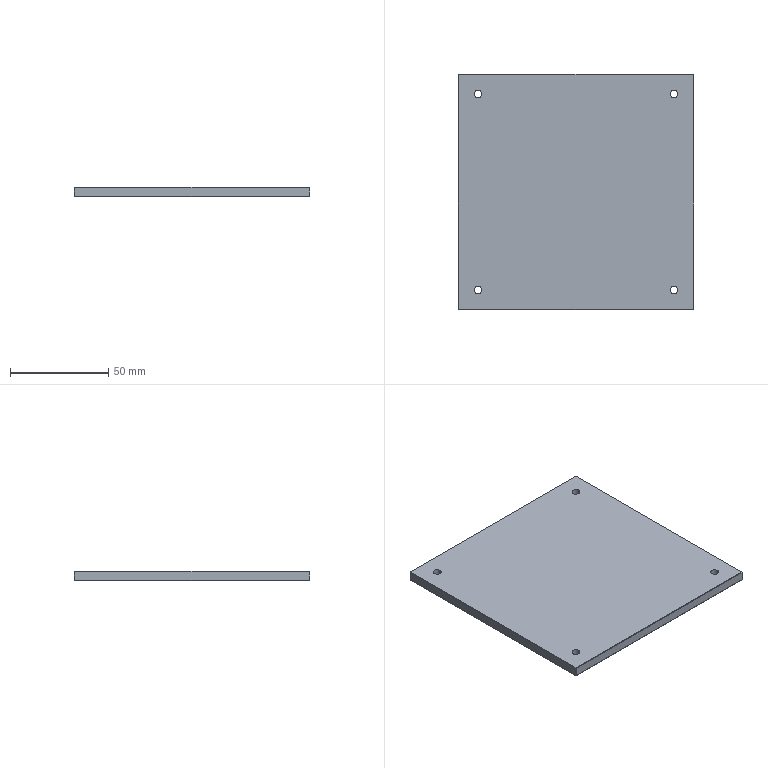Part | NX | 1 solid | 26 faces | box 120 x 120 x 5 mm | volume 71705 mm3 | plane 18 | cylinder 8 | commonest cylinder face diameters 4 x8
STEP:
#1=CARTESIAN_POINT('',(-59.7,-59.7,0.));
#2=VERTEX_POINT('',#1);
#3=CARTESIAN_POINT('',(-59.7,59.7,0.));
#4=VERTEX_POINT('',#3);
#5=CARTESIAN_POINT('',(-59.7,0.,0.));
#6=DIRECTION('',(0.,1.,0.));
#7=VECTOR('',#6,1000.);
#8=LINE('',#5,#7);
#9=EDGE_CURVE('',#2,#4,#8,.T.);
#10=ORIENTED_EDGE('',*,*,#9,.T.);
#11=CARTESIAN_POINT('',(59.7,59.7,0.));
#12=VERTEX_POINT('',#11);
#13=CARTESIAN_POINT('',(0.,59.7,0.));
#14=DIRECTION('',(1.,0.,0.));
#15=VECTOR('',#14,1000.);
#16=LINE('',#13,#15);
#17=EDGE_CURVE('',#4,#12,#16,.T.);
#18=ORIENTED_EDGE('',*,*,#17,.T.);
#19=CARTESIAN_POINT('',(59.7,-59.7,0.));
#20=VERTEX_POINT('',#19);
#21=CARTESIAN_POINT('',(59.7,0.,0.));
#22=DIRECTION('',(0.,-1.,0.));
#23=VECTOR('',#22,1000.);
#24=LINE('',#21,#23);
#25=EDGE_CURVE('',#12,#20,#24,.T.);
#26=ORIENTED_EDGE('',*,*,#25,.T.);
#27=CARTESIAN_POINT('',(0.,-59.7,0.));
#28=DIRECTION('',(-1.,0.,0.));
#29=VECTOR('',#28,1000.);
#30=LINE('',#27,#29);
#31=EDGE_CURVE('',#20,#2,#30,.T.);
#32=ORIENTED_EDGE('',*,*,#31,.T.);
#33=EDGE_LOOP('',(#10,#18,#26,#32));
#34=FACE_BOUND('',#33,.T.);
#35=CARTESIAN_POINT('',(52.,50.,0.));
#36=VERTEX_POINT('',#35);
#37=CARTESIAN_POINT('',(48.,50.,0.));
#38=VERTEX_POINT('',#37);
#39=CARTESIAN_POINT('',(50.,50.,0.));
#40=DIRECTION('',(0.,0.,-1.));
#41=DIRECTION('',(-1.,0.,0.));
#42=AXIS2_PLACEMENT_3D('',#39,#40,#41);
#43=CIRCLE('',#42,2.);
#44=EDGE_CURVE('',#36,#38,#43,.T.);
#45=ORIENTED_EDGE('',*,*,#44,.F.);
#46=CARTESIAN_POINT('',(50.,50.,0.));
#47=DIRECTION('',(0.,0.,-1.));
#48=DIRECTION('',(-1.,0.,0.));
#49=AXIS2_PLACEMENT_3D('',#46,#47,#48);
#50=CIRCLE('',#49,2.);
#51=EDGE_CURVE('',#38,#36,#50,.T.);
#52=ORIENTED_EDGE('',*,*,#51,.F.);
#53=EDGE_LOOP('',(#45,#52));
#54=FACE_BOUND('',#53,.T.);
#55=CARTESIAN_POINT('',(-48.,-50.,0.));
#56=VERTEX_POINT('',#55);
#57=CARTESIAN_POINT('',(-52.,-50.,0.));
#58=VERTEX_POINT('',#57);
#59=CARTESIAN_POINT('',(-50.,-50.,0.));
#60=DIRECTION('',(0.,0.,-1.));
#61=DIRECTION('',(-1.,0.,0.));
#62=AXIS2_PLACEMENT_3D('',#59,#60,#61);
#63=CIRCLE('',#62,2.);
#64=EDGE_CURVE('',#56,#58,#63,.T.);
#65=ORIENTED_EDGE('',*,*,#64,.F.);
#66=CARTESIAN_POINT('',(-50.,-50.,0.));
#67=DIRECTION('',(0.,0.,-1.));
#68=DIRECTION('',(-1.,0.,0.));
#69=AXIS2_PLACEMENT_3D('',#66,#67,#68);
#70=CIRCLE('',#69,2.);
#71=EDGE_CURVE('',#58,#56,#70,.T.);
#72=ORIENTED_EDGE('',*,*,#71,.F.);
#73=EDGE_LOOP('',(#65,#72));
#74=FACE_BOUND('',#73,.T.);
#75=CARTESIAN_POINT('',(-48.,50.,0.));
#76=VERTEX_POINT('',#75);
#77=CARTESIAN_POINT('',(-52.,50.,0.));
#78=VERTEX_POINT('',#77);
#79=CARTESIAN_POINT('',(-50.,50.,0.));
#80=DIRECTION('',(0.,0.,-1.));
#81=DIRECTION('',(-1.,0.,0.));
#82=AXIS2_PLACEMENT_3D('',#79,#80,#81);
#83=CIRCLE('',#82,2.);
#84=EDGE_CURVE('',#76,#78,#83,.T.);
#85=ORIENTED_EDGE('',*,*,#84,.F.);
#86=CARTESIAN_POINT('',(-50.,50.,0.));
#87=DIRECTION('',(0.,0.,-1.));
#88=DIRECTION('',(-1.,0.,0.));
#89=AXIS2_PLACEMENT_3D('',#86,#87,#88);
#90=CIRCLE('',#89,2.);
#91=EDGE_CURVE('',#78,#76,#90,.T.);
#92=ORIENTED_EDGE('',*,*,#91,.F.);
#93=EDGE_LOOP('',(#85,#92));
#94=FACE_BOUND('',#93,.T.);
#95=CARTESIAN_POINT('',(52.,-50.,0.));
#96=VERTEX_POINT('',#95);
#97=CARTESIAN_POINT('',(48.,-50.,0.));
#98=VERTEX_POINT('',#97);
#99=CARTESIAN_POINT('',(50.,-50.,0.));
#100=DIRECTION('',(0.,0.,-1.));
#101=DIRECTION('',(-1.,0.,0.));
#102=AXIS2_PLACEMENT_3D('',#99,#100,#101);
#103=CIRCLE('',#102,2.);
#104=EDGE_CURVE('',#96,#98,#103,.T.);
#105=ORIENTED_EDGE('',*,*,#104,.F.);
#106=CARTESIAN_POINT('',(50.,-50.,0.));
#107=DIRECTION('',(0.,0.,-1.));
#108=DIRECTION('',(-1.,0.,0.));
#109=AXIS2_PLACEMENT_3D('',#106,#107,#108);
#110=CIRCLE('',#109,2.);
#111=EDGE_CURVE('',#98,#96,#110,.T.);
#112=ORIENTED_EDGE('',*,*,#111,.F.);
#113=EDGE_LOOP('',(#105,#112));
#114=FACE_BOUND('',#113,.T.);
#115=CARTESIAN_POINT('',(0.,0.,0.));
#116=DIRECTION('',(0.,0.,1.));
#117=DIRECTION('',(1.,0.,0.));
#118=AXIS2_PLACEMENT_3D('',#115,#116,#117);
#119=PLANE('',#118);
#120=ADVANCED_FACE('',(#34,#54,#74,#94,#114),#119,.F.);
#121=CARTESIAN_POINT('',(-60.,59.7,4.7));
#122=VERTEX_POINT('',#121);
#123=CARTESIAN_POINT('',(-60.,59.7,0.3));
#124=VERTEX_POINT('',#123);
#125=CARTESIAN_POINT('',(-60.,59.7,2.5));
#126=DIRECTION('',(0.,0.,-1.));
#127=VECTOR('',#126,1000.);
#128=LINE('',#125,#127);
#129=EDGE_CURVE('',#122,#124,#128,.T.);
#130=ORIENTED_EDGE('',*,*,#129,.T.);
#131=CARTESIAN_POINT('',(-60.,-59.7,0.3));
#132=VERTEX_POINT('',#131);
#133=CARTESIAN_POINT('',(-60.,0.,0.3));
#134=DIRECTION('',(0.,1.,0.));
#135=VECTOR('',#134,1000.);
#136=LINE('',#133,#135);
#137=EDGE_CURVE('',#132,#124,#136,.T.);
#138=ORIENTED_EDGE('',*,*,#137,.F.);
#139=CARTESIAN_POINT('',(-60.,-59.7,4.7));
#140=VERTEX_POINT('',#139);
#141=CARTESIAN_POINT('',(-60.,-59.7,2.5));
#142=DIRECTION('',(0.,0.,-1.));
#143=VECTOR('',#142,1000.);
#144=LINE('',#141,#143);
#145=EDGE_CURVE('',#140,#132,#144,.T.);
#146=ORIENTED_EDGE('',*,*,#145,.F.);
#147=CARTESIAN_POINT('',(-60.,0.,4.7));
#148=DIRECTION('',(0.,1.,0.));
#149=VECTOR('',#148,1000.);
#150=LINE('',#147,#149);
#151=EDGE_CURVE('',#140,#122,#150,.T.);
#152=ORIENTED_EDGE('',*,*,#151,.T.);
#153=EDGE_LOOP('',(#130,#138,#146,#152));
#154=FACE_BOUND('',#153,.T.);
#155=CARTESIAN_POINT('',(-60.,60.,0.));
#156=DIRECTION('',(-1.,0.,0.));
#157=DIRECTION('',(0.,0.,1.));
#158=AXIS2_PLACEMENT_3D('',#155,#156,#157);
#159=PLANE('',#158);
#160=ADVANCED_FACE('',(#154),#159,.T.);
#161=CARTESIAN_POINT('',(59.7,60.,4.7));
#162=VERTEX_POINT('',#161);
#163=CARTESIAN_POINT('',(59.7,60.,0.3));
#164=VERTEX_POINT('',#163);
#165=CARTESIAN_POINT('',(59.7,60.,2.5));
#166=DIRECTION('',(0.,0.,-1.));
#167=VECTOR('',#166,1000.);
#168=LINE('',#165,#167);
#169=EDGE_CURVE('',#162,#164,#168,.T.);
#170=ORIENTED_EDGE('',*,*,#169,.T.);
#171=CARTESIAN_POINT('',(-59.7,60.,0.3));
#172=VERTEX_POINT('',#171);
#173=CARTESIAN_POINT('',(0.,60.,0.3));
#174=DIRECTION('',(1.,0.,0.));
#175=VECTOR('',#174,1000.);
#176=LINE('',#173,#175);
#177=EDGE_CURVE('',#172,#164,#176,.T.);
#178=ORIENTED_EDGE('',*,*,#177,.F.);
#179=CARTESIAN_POINT('',(-59.7,60.,4.7));
#180=VERTEX_POINT('',#179);
#181=CARTESIAN_POINT('',(-59.7,60.,2.5));
#182=DIRECTION('',(0.,0.,-1.));
#183=VECTOR('',#182,1000.);
#184=LINE('',#181,#183);
#185=EDGE_CURVE('',#180,#172,#184,.T.);
#186=ORIENTED_EDGE('',*,*,#185,.F.);
#187=CARTESIAN_POINT('',(0.,60.,4.7));
#188=DIRECTION('',(1.,0.,0.));
#189=VECTOR('',#188,1000.);
#190=LINE('',#187,#189);
#191=EDGE_CURVE('',#180,#162,#190,.T.);
#192=ORIENTED_EDGE('',*,*,#191,.T.);
#193=EDGE_LOOP('',(#170,#178,#186,#192));
#194=FACE_BOUND('',#193,.T.);
#195=CARTESIAN_POINT('',(60.,60.,0.));
#196=DIRECTION('',(0.,1.,0.));
#197=DIRECTION('',(1.,0.,0.));
#198=AXIS2_PLACEMENT_3D('',#195,#196,#197);
#199=PLANE('',#198);
#200=ADVANCED_FACE('',(#194),#199,.T.);
#201=CARTESIAN_POINT('',(60.,-59.7,4.7));
#202=VERTEX_POINT('',#201);
#203=CARTESIAN_POINT('',(60.,-59.7,0.3));
#204=VERTEX_POINT('',#203);
#205=CARTESIAN_POINT('',(60.,-59.7,2.5));
#206=DIRECTION('',(0.,0.,-1.));
#207=VECTOR('',#206,1000.);
#208=LINE('',#205,#207);
#209=EDGE_CURVE('',#202,#204,#208,.T.);
#210=ORIENTED_EDGE('',*,*,#209,.T.);
#211=CARTESIAN_POINT('',(60.,59.7,0.3));
#212=VERTEX_POINT('',#211);
#213=CARTESIAN_POINT('',(60.,0.,0.3));
#214=DIRECTION('',(0.,-1.,0.));
#215=VECTOR('',#214,1000.);
#216=LINE('',#213,#215);
#217=EDGE_CURVE('',#212,#204,#216,.T.);
#218=ORIENTED_EDGE('',*,*,#217,.F.);
#219=CARTESIAN_POINT('',(60.,59.7,4.7));
#220=VERTEX_POINT('',#219);
#221=CARTESIAN_POINT('',(60.,59.7,2.5));
#222=DIRECTION('',(0.,0.,-1.));
#223=VECTOR('',#222,1000.);
#224=LINE('',#221,#223);
#225=EDGE_CURVE('',#220,#212,#224,.T.);
#226=ORIENTED_EDGE('',*,*,#225,.F.);
#227=CARTESIAN_POINT('',(60.,0.,4.7));
#228=DIRECTION('',(0.,-1.,0.));
#229=VECTOR('',#228,1000.);
#230=LINE('',#227,#229);
#231=EDGE_CURVE('',#220,#202,#230,.T.);
#232=ORIENTED_EDGE('',*,*,#231,.T.);
#233=EDGE_LOOP('',(#210,#218,#226,#232));
#234=FACE_BOUND('',#233,.T.);
#235=CARTESIAN_POINT('',(60.,-60.,0.));
#236=DIRECTION('',(1.,0.,0.));
#237=DIRECTION('',(0.,1.,0.));
#238=AXIS2_PLACEMENT_3D('',#235,#236,#237);
#239=PLANE('',#238);
#240=ADVANCED_FACE('',(#234),#239,.T.);
#241=CARTESIAN_POINT('',(59.7,-60.,4.7));
#242=VERTEX_POINT('',#241);
#243=CARTESIAN_POINT('',(-59.7,-60.,4.7));
#244=VERTEX_POINT('',#243);
#245=CARTESIAN_POINT('',(0.,-60.,4.7));
#246=DIRECTION('',(-1.,0.,0.));
#247=VECTOR('',#246,1000.);
#248=LINE('',#245,#247);
#249=EDGE_CURVE('',#242,#244,#248,.T.);
#250=ORIENTED_EDGE('',*,*,#249,.T.);
#251=CARTESIAN_POINT('',(-59.7,-60.,0.3));
#252=VERTEX_POINT('',#251);
#253=CARTESIAN_POINT('',(-59.7,-60.,2.5));
#254=DIRECTION('',(0.,0.,-1.));
#255=VECTOR('',#254,1000.);
#256=LINE('',#253,#255);
#257=EDGE_CURVE('',#244,#252,#256,.T.);
#258=ORIENTED_EDGE('',*,*,#257,.T.);
#259=CARTESIAN_POINT('',(59.7,-60.,0.3));
#260=VERTEX_POINT('',#259);
#261=CARTESIAN_POINT('',(0.,-60.,0.3));
#262=DIRECTION('',(-1.,0.,0.));
#263=VECTOR('',#262,1000.);
#264=LINE('',#261,#263);
#265=EDGE_CURVE('',#260,#252,#264,.T.);
#266=ORIENTED_EDGE('',*,*,#265,.F.);
#267=CARTESIAN_POINT('',(59.7,-60.,2.5));
#268=DIRECTION('',(0.,0.,-1.));
#269=VECTOR('',#268,1000.);
#270=LINE('',#267,#269);
#271=EDGE_CURVE('',#242,#260,#270,.T.);
#272=ORIENTED_EDGE('',*,*,#271,.F.);
#273=EDGE_LOOP('',(#250,#258,#266,#272));
#274=FACE_BOUND('',#273,.T.);
#275=CARTESIAN_POINT('',(-60.,-60.,0.));
#276=DIRECTION('',(0.,-1.,0.));
#277=DIRECTION('',(0.,0.,-1.));
#278=AXIS2_PLACEMENT_3D('',#275,#276,#277);
#279=PLANE('',#278);
#280=ADVANCED_FACE('',(#274),#279,.T.);
#281=CARTESIAN_POINT('',(-59.7,-59.7,5.));
#282=VERTEX_POINT('',#281);
#283=CARTESIAN_POINT('',(-59.7,59.7,5.));
#284=VERTEX_POINT('',#283);
#285=CARTESIAN_POINT('',(-59.7,0.,5.));
#286=DIRECTION('',(0.,1.,0.));
#287=VECTOR('',#286,1000.);
#288=LINE('',#285,#287);
#289=EDGE_CURVE('',#282,#284,#288,.T.);
#290=ORIENTED_EDGE('',*,*,#289,.F.);
#291=CARTESIAN_POINT('',(59.7,-59.7,5.));
#292=VERTEX_POINT('',#291);
#293=CARTESIAN_POINT('',(0.,-59.7,5.));
#294=DIRECTION('',(-1.,0.,0.));
#295=VECTOR('',#294,1000.);
#296=LINE('',#293,#295);
#297=EDGE_CURVE('',#292,#282,#296,.T.);
#298=ORIENTED_EDGE('',*,*,#297,.F.);
#299=CARTESIAN_POINT('',(59.7,59.7,5.));
#300=VERTEX_POINT('',#299);
#301=CARTESIAN_POINT('',(59.7,0.,5.));
#302=DIRECTION('',(0.,-1.,0.));
#303=VECTOR('',#302,1000.);
#304=LINE('',#301,#303);
#305=EDGE_CURVE('',#300,#292,#304,.T.);
#306=ORIENTED_EDGE('',*,*,#305,.F.);
#307=CARTESIAN_POINT('',(0.,59.7,5.));
#308=DIRECTION('',(1.,0.,0.));
#309=VECTOR('',#308,1000.);
#310=LINE('',#307,#309);
#311=EDGE_CURVE('',#284,#300,#310,.T.);
#312=ORIENTED_EDGE('',*,*,#311,.F.);
#313=EDGE_LOOP('',(#290,#298,#306,#312));
#314=FACE_BOUND('',#313,.T.);
#315=CARTESIAN_POINT('',(52.,50.,5.));
#316=VERTEX_POINT('',#315);
#317=CARTESIAN_POINT('',(48.,50.,5.));
#318=VERTEX_POINT('',#317);
#319=CARTESIAN_POINT('',(50.,50.,5.));
#320=DIRECTION('',(0.,0.,-1.));
#321=DIRECTION('',(-1.,0.,0.));
#322=AXIS2_PLACEMENT_3D('',#319,#320,#321);
#323=CIRCLE('',#322,2.);
#324=EDGE_CURVE('',#316,#318,#323,.T.);
#325=ORIENTED_EDGE('',*,*,#324,.T.);
#326=CARTESIAN_POINT('',(50.,50.,5.));
#327=DIRECTION('',(0.,0.,-1.));
#328=DIRECTION('',(-1.,0.,0.));
#329=AXIS2_PLACEMENT_3D('',#326,#327,#328);
#330=CIRCLE('',#329,2.);
#331=EDGE_CURVE('',#318,#316,#330,.T.);
#332=ORIENTED_EDGE('',*,*,#331,.T.);
#333=EDGE_LOOP('',(#325,#332));
#334=FACE_BOUND('',#333,.T.);
#335=CARTESIAN_POINT('',(-48.,-50.,5.));
#336=VERTEX_POINT('',#335);
#337=CARTESIAN_POINT('',(-52.,-50.,5.));
#338=VERTEX_POINT('',#337);
#339=CARTESIAN_POINT('',(-50.,-50.,5.));
#340=DIRECTION('',(0.,0.,-1.));
#341=DIRECTION('',(-1.,0.,0.));
#342=AXIS2_PLACEMENT_3D('',#339,#340,#341);
#343=CIRCLE('',#342,2.);
#344=EDGE_CURVE('',#336,#338,#343,.T.);
#345=ORIENTED_EDGE('',*,*,#344,.T.);
#346=CARTESIAN_POINT('',(-50.,-50.,5.));
#347=DIRECTION('',(0.,0.,-1.));
#348=DIRECTION('',(-1.,0.,0.));
#349=AXIS2_PLACEMENT_3D('',#346,#347,#348);
#350=CIRCLE('',#349,2.);
#351=EDGE_CURVE('',#338,#336,#350,.T.);
#352=ORIENTED_EDGE('',*,*,#351,.T.);
#353=EDGE_LOOP('',(#345,#352));
#354=FACE_BOUND('',#353,.T.);
#355=CARTESIAN_POINT('',(-48.,50.,5.));
#356=VERTEX_POINT('',#355);
#357=CARTESIAN_POINT('',(-52.,50.,5.));
#358=VERTEX_POINT('',#357);
#359=CARTESIAN_POINT('',(-50.,50.,5.));
#360=DIRECTION('',(0.,0.,-1.));
#361=DIRECTION('',(-1.,0.,0.));
#362=AXIS2_PLACEMENT_3D('',#359,#360,#361);
#363=CIRCLE('',#362,2.);
#364=EDGE_CURVE('',#356,#358,#363,.T.);
#365=ORIENTED_EDGE('',*,*,#364,.T.);
#366=CARTESIAN_POINT('',(-50.,50.,5.));
#367=DIRECTION('',(0.,0.,-1.));
#368=DIRECTION('',(-1.,0.,0.));
#369=AXIS2_PLACEMENT_3D('',#366,#367,#368);
#370=CIRCLE('',#369,2.);
#371=EDGE_CURVE('',#358,#356,#370,.T.);
#372=ORIENTED_EDGE('',*,*,#371,.T.);
#373=EDGE_LOOP('',(#365,#372));
#374=FACE_BOUND('',#373,.T.);
#375=CARTESIAN_POINT('',(52.,-50.,5.));
#376=VERTEX_POINT('',#375);
#377=CARTESIAN_POINT('',(48.,-50.,5.));
#378=VERTEX_POINT('',#377);
#379=CARTESIAN_POINT('',(50.,-50.,5.));
#380=DIRECTION('',(0.,0.,-1.));
#381=DIRECTION('',(-1.,0.,0.));
#382=AXIS2_PLACEMENT_3D('',#379,#380,#381);
#383=CIRCLE('',#382,2.);
#384=EDGE_CURVE('',#376,#378,#383,.T.);
#385=ORIENTED_EDGE('',*,*,#384,.T.);
#386=CARTESIAN_POINT('',(50.,-50.,5.));
#387=DIRECTION('',(0.,0.,-1.));
#388=DIRECTION('',(-1.,0.,0.));
#389=AXIS2_PLACEMENT_3D('',#386,#387,#388);
#390=CIRCLE('',#389,2.);
#391=EDGE_CURVE('',#378,#376,#390,.T.);
#392=ORIENTED_EDGE('',*,*,#391,.T.);
#393=EDGE_LOOP('',(#385,#392));
#394=FACE_BOUND('',#393,.T.);
#395=CARTESIAN_POINT('',(0.,0.,5.));
#396=DIRECTION('',(0.,0.,1.));
#397=DIRECTION('',(1.,0.,0.));
#398=AXIS2_PLACEMENT_3D('',#395,#396,#397);
#399=PLANE('',#398);
#400=ADVANCED_FACE('',(#314,#334,#354,#374,#394),#399,.T.);
#401=ORIENTED_EDGE('',*,*,#384,.F.);
#402=CARTESIAN_POINT('',(52.,-50.,5.));
#403=DIRECTION('',(0.,0.,-1.));
#404=VECTOR('',#403,1000.);
#405=LINE('',#402,#404);
#406=EDGE_CURVE('',#96,#376,#405,.F.);
#407=ORIENTED_EDGE('',*,*,#406,.F.);
#408=ORIENTED_EDGE('',*,*,#104,.T.);
#409=CARTESIAN_POINT('',(48.,-50.,5.));
#410=DIRECTION('',(0.,0.,-1.));
#411=VECTOR('',#410,1000.);
#412=LINE('',#409,#411);
#413=EDGE_CURVE('',#98,#378,#412,.F.);
#414=ORIENTED_EDGE('',*,*,#413,.T.);
#415=EDGE_LOOP('',(#401,#407,#408,#414));
#416=FACE_BOUND('',#415,.T.);
#417=CARTESIAN_POINT('',(50.,-50.,5.));
#418=DIRECTION('',(0.,0.,-1.));
#419=DIRECTION('',(-1.,0.,0.));
#420=AXIS2_PLACEMENT_3D('',#417,#418,#419);
#421=CYLINDRICAL_SURFACE('',#420,2.);
#422=ADVANCED_FACE('',(#416),#421,.F.);
#423=ORIENTED_EDGE('',*,*,#64,.T.);
#424=CARTESIAN_POINT('',(-52.,-50.,5.));
#425=DIRECTION('',(0.,0.,-1.));
#426=VECTOR('',#425,1000.);
#427=LINE('',#424,#426);
#428=EDGE_CURVE('',#58,#338,#427,.F.);
#429=ORIENTED_EDGE('',*,*,#428,.T.);
#430=ORIENTED_EDGE('',*,*,#344,.F.);
#431=CARTESIAN_POINT('',(-48.,-50.,5.));
#432=DIRECTION('',(0.,0.,-1.));
#433=VECTOR('',#432,1000.);
#434=LINE('',#431,#433);
#435=EDGE_CURVE('',#56,#336,#434,.F.);
#436=ORIENTED_EDGE('',*,*,#435,.F.);
#437=EDGE_LOOP('',(#423,#429,#430,#436));
#438=FACE_BOUND('',#437,.T.);
#439=CARTESIAN_POINT('',(-50.,-50.,5.));
#440=DIRECTION('',(0.,0.,-1.));
#441=DIRECTION('',(-1.,0.,0.));
#442=AXIS2_PLACEMENT_3D('',#439,#440,#441);
#443=CYLINDRICAL_SURFACE('',#442,2.);
#444=ADVANCED_FACE('',(#438),#443,.F.);
#445=ORIENTED_EDGE('',*,*,#44,.T.);
#446=CARTESIAN_POINT('',(48.,50.,5.));
#447=DIRECTION('',(0.,0.,-1.));
#448=VECTOR('',#447,1000.);
#449=LINE('',#446,#448);
#450=EDGE_CURVE('',#38,#318,#449,.F.);
#451=ORIENTED_EDGE('',*,*,#450,.T.);
#452=ORIENTED_EDGE('',*,*,#324,.F.);
#453=CARTESIAN_POINT('',(52.,50.,5.));
#454=DIRECTION('',(0.,0.,-1.));
#455=VECTOR('',#454,1000.);
#456=LINE('',#453,#455);
#457=EDGE_CURVE('',#36,#316,#456,.F.);
#458=ORIENTED_EDGE('',*,*,#457,.F.);
#459=EDGE_LOOP('',(#445,#451,#452,#458));
#460=FACE_BOUND('',#459,.T.);
#461=CARTESIAN_POINT('',(50.,50.,5.));
#462=DIRECTION('',(0.,0.,-1.));
#463=DIRECTION('',(-1.,0.,0.));
#464=AXIS2_PLACEMENT_3D('',#461,#462,#463);
#465=CYLINDRICAL_SURFACE('',#464,2.);
#466=ADVANCED_FACE('',(#460),#465,.F.);
#467=ORIENTED_EDGE('',*,*,#84,.T.);
#468=CARTESIAN_POINT('',(-52.,50.,5.));
#469=DIRECTION('',(0.,0.,-1.));
#470=VECTOR('',#469,1000.);
#471=LINE('',#468,#470);
#472=EDGE_CURVE('',#78,#358,#471,.F.);
#473=ORIENTED_EDGE('',*,*,#472,.T.);
#474=ORIENTED_EDGE('',*,*,#364,.F.);
#475=CARTESIAN_POINT('',(-48.,50.,5.));
#476=DIRECTION('',(0.,0.,-1.));
#477=VECTOR('',#476,1000.);
#478=LINE('',#475,#477);
#479=EDGE_CURVE('',#76,#356,#478,.F.);
#480=ORIENTED_EDGE('',*,*,#479,.F.);
#481=EDGE_LOOP('',(#467,#473,#474,#480));
#482=FACE_BOUND('',#481,.T.);
#483=CARTESIAN_POINT('',(-50.,50.,5.));
#484=DIRECTION('',(0.,0.,-1.));
#485=DIRECTION('',(-1.,0.,0.));
#486=AXIS2_PLACEMENT_3D('',#483,#484,#485);
#487=CYLINDRICAL_SURFACE('',#486,2.);
#488=ADVANCED_FACE('',(#482),#487,.F.);
#489=ORIENTED_EDGE('',*,*,#191,.F.);
#490=CARTESIAN_POINT('',(-59.85,59.85,4.85));
#491=VERTEX_POINT('',#490);
#492=CARTESIAN_POINT('',(-55.,64.7,0.));
#493=DIRECTION('',(-0.5774,-0.5774,0.5774));
#494=VECTOR('',#493,1000.);
#495=LINE('',#492,#494);
#496=EDGE_CURVE('',#180,#491,#495,.T.);
#497=ORIENTED_EDGE('',*,*,#496,.T.);
#498=CARTESIAN_POINT('',(-64.7,64.7,0.));
#499=DIRECTION('',(0.5774,-0.5774,0.5774));
#500=VECTOR('',#499,1000.);
#501=LINE('',#498,#500);
#502=EDGE_CURVE('',#491,#284,#501,.T.);
#503=ORIENTED_EDGE('',*,*,#502,.T.);
#504=ORIENTED_EDGE('',*,*,#311,.T.);
#505=CARTESIAN_POINT('',(59.85,59.85,4.85));
#506=VERTEX_POINT('',#505);
#507=CARTESIAN_POINT('',(64.7,64.7,0.));
#508=DIRECTION('',(0.5774,0.5774,-0.5774));
#509=VECTOR('',#508,1000.);
#510=LINE('',#507,#509);
#511=EDGE_CURVE('',#300,#506,#510,.T.);
#512=ORIENTED_EDGE('',*,*,#511,.T.);
#513=CARTESIAN_POINT('',(55.,64.7,0.));
#514=DIRECTION('',(-0.5774,0.5774,-0.5774));
#515=VECTOR('',#514,1000.);
#516=LINE('',#513,#515);
#517=EDGE_CURVE('',#506,#162,#516,.T.);
#518=ORIENTED_EDGE('',*,*,#517,.T.);
#519=EDGE_LOOP('',(#489,#497,#503,#504,#512,#518));
#520=FACE_BOUND('',#519,.T.);
#521=CARTESIAN_POINT('',(0.,59.85,4.85));
#522=DIRECTION('',(0.,0.7071,0.7071));
#523=DIRECTION('',(1.,0.,0.));
#524=AXIS2_PLACEMENT_3D('',#521,#522,#523);
#525=PLANE('',#524);
#526=ADVANCED_FACE('',(#520),#525,.T.);
#527=ORIENTED_EDGE('',*,*,#17,.F.);
#528=CARTESIAN_POINT('',(-59.85,59.85,0.15));
#529=VERTEX_POINT('',#528);
#530=CARTESIAN_POINT('',(-59.7,59.7,0.));
#531=DIRECTION('',(-0.5774,0.5774,0.5774));
#532=VECTOR('',#531,1000.);
#533=LINE('',#530,#532);
#534=EDGE_CURVE('',#4,#529,#533,.T.);
#535=ORIENTED_EDGE('',*,*,#534,.T.);
#536=CARTESIAN_POINT('',(-60.,59.7,0.));
#537=DIRECTION('',(0.5774,0.5774,0.5774));
#538=VECTOR('',#537,1000.);
#539=LINE('',#536,#538);
#540=EDGE_CURVE('',#529,#172,#539,.T.);
#541=ORIENTED_EDGE('',*,*,#540,.T.);
#542=ORIENTED_EDGE('',*,*,#177,.T.);
#543=CARTESIAN_POINT('',(59.85,59.85,0.15));
#544=VERTEX_POINT('',#543);
#545=CARTESIAN_POINT('',(60.,59.7,0.));
#546=DIRECTION('',(0.5774,-0.5774,-0.5774));
#547=VECTOR('',#546,1000.);
#548=LINE('',#545,#547);
#549=EDGE_CURVE('',#164,#544,#548,.T.);
#550=ORIENTED_EDGE('',*,*,#549,.T.);
#551=CARTESIAN_POINT('',(59.7,59.7,0.));
#552=DIRECTION('',(-0.5774,-0.5774,-0.5774));
#553=VECTOR('',#552,1000.);
#554=LINE('',#551,#553);
#555=EDGE_CURVE('',#544,#12,#554,.T.);
#556=ORIENTED_EDGE('',*,*,#555,.T.);
#557=EDGE_LOOP('',(#527,#535,#541,#542,#550,#556));
#558=FACE_BOUND('',#557,.T.);
#559=CARTESIAN_POINT('',(0.,59.85,0.15));
#560=DIRECTION('',(0.,0.7071,-0.7071));
#561=DIRECTION('',(-1.,0.,0.));
#562=AXIS2_PLACEMENT_3D('',#559,#560,#561);
#563=PLANE('',#562);
#564=ADVANCED_FACE('',(#558),#563,.T.);
#565=ORIENTED_EDGE('',*,*,#25,.F.);
#566=ORIENTED_EDGE('',*,*,#555,.F.);
#567=CARTESIAN_POINT('',(59.7,60.,0.));
#568=DIRECTION('',(0.5774,-0.5774,0.5774));
#569=VECTOR('',#568,1000.);
#570=LINE('',#567,#569);
#571=EDGE_CURVE('',#544,#212,#570,.T.);
#572=ORIENTED_EDGE('',*,*,#571,.T.);
#573=ORIENTED_EDGE('',*,*,#217,.T.);
#574=CARTESIAN_POINT('',(59.85,-59.85,0.15));
#575=VERTEX_POINT('',#574);
#576=CARTESIAN_POINT('',(59.7,-60.,0.));
#577=DIRECTION('',(-0.5774,-0.5774,-0.5774));
#578=VECTOR('',#577,1000.);
#579=LINE('',#576,#578);
#580=EDGE_CURVE('',#204,#575,#579,.T.);
#581=ORIENTED_EDGE('',*,*,#580,.T.);
#582=CARTESIAN_POINT('',(59.7,-59.7,0.));
#583=DIRECTION('',(-0.5774,0.5774,-0.5774));
#584=VECTOR('',#583,1000.);
#585=LINE('',#582,#584);
#586=EDGE_CURVE('',#575,#20,#585,.T.);
#587=ORIENTED_EDGE('',*,*,#586,.T.);
#588=EDGE_LOOP('',(#565,#566,#572,#573,#581,#587));
#589=FACE_BOUND('',#588,.T.);
#590=CARTESIAN_POINT('',(59.85,0.,0.15));
#591=DIRECTION('',(0.7071,0.,-0.7071));
#592=DIRECTION('',(0.,-1.,0.));
#593=AXIS2_PLACEMENT_3D('',#590,#591,#592);
#594=PLANE('',#593);
#595=ADVANCED_FACE('',(#589),#594,.T.);
#596=ORIENTED_EDGE('',*,*,#169,.F.);
#597=ORIENTED_EDGE('',*,*,#517,.F.);
#598=CARTESIAN_POINT('',(64.7,55.,0.));
#599=DIRECTION('',(0.5774,-0.5774,-0.5774));
#600=VECTOR('',#599,1000.);
#601=LINE('',#598,#600);
#602=EDGE_CURVE('',#506,#220,#601,.T.);
#603=ORIENTED_EDGE('',*,*,#602,.T.);
#604=ORIENTED_EDGE('',*,*,#225,.T.);
#605=ORIENTED_EDGE('',*,*,#571,.F.);
#606=ORIENTED_EDGE('',*,*,#549,.F.);
#607=EDGE_LOOP('',(#596,#597,#603,#604,#605,#606));
#608=FACE_BOUND('',#607,.T.);
#609=CARTESIAN_POINT('',(59.85,59.85,2.5));
#610=DIRECTION('',(0.7071,0.7071,0.));
#611=DIRECTION('',(0.,0.,-1.));
#612=AXIS2_PLACEMENT_3D('',#609,#610,#611);
#613=PLANE('',#612);
#614=ADVANCED_FACE('',(#608),#613,.T.);
#615=ORIENTED_EDGE('',*,*,#231,.F.);
#616=ORIENTED_EDGE('',*,*,#602,.F.);
#617=ORIENTED_EDGE('',*,*,#511,.F.);
#618=ORIENTED_EDGE('',*,*,#305,.T.);
#619=CARTESIAN_POINT('',(59.85,-59.85,4.85));
#620=VERTEX_POINT('',#619);
#621=CARTESIAN_POINT('',(64.7,-64.7,0.));
#622=DIRECTION('',(0.5774,-0.5774,-0.5774));
#623=VECTOR('',#622,1000.);
#624=LINE('',#621,#623);
#625=EDGE_CURVE('',#292,#620,#624,.T.);
#626=ORIENTED_EDGE('',*,*,#625,.T.);
#627=CARTESIAN_POINT('',(64.7,-55.,0.));
#628=DIRECTION('',(0.5774,0.5774,-0.5774));
#629=VECTOR('',#628,1000.);
#630=LINE('',#627,#629);
#631=EDGE_CURVE('',#620,#202,#630,.T.);
#632=ORIENTED_EDGE('',*,*,#631,.T.);
#633=EDGE_LOOP('',(#615,#616,#617,#618,#626,#632));
#634=FACE_BOUND('',#633,.T.);
#635=CARTESIAN_POINT('',(59.85,0.,4.85));
#636=DIRECTION('',(0.7071,0.,0.7071));
#637=DIRECTION('',(0.,-1.,0.));
#638=AXIS2_PLACEMENT_3D('',#635,#636,#637);
#639=PLANE('',#638);
#640=ADVANCED_FACE('',(#634),#639,.T.);
#641=ORIENTED_EDGE('',*,*,#209,.F.);
#642=ORIENTED_EDGE('',*,*,#631,.F.);
#643=CARTESIAN_POINT('',(55.,-64.7,0.));
#644=DIRECTION('',(-0.5774,-0.5774,-0.5774));
#645=VECTOR('',#644,1000.);
#646=LINE('',#643,#645);
#647=EDGE_CURVE('',#620,#242,#646,.T.);
#648=ORIENTED_EDGE('',*,*,#647,.T.);
#649=ORIENTED_EDGE('',*,*,#271,.T.);
#650=CARTESIAN_POINT('',(60.,-59.7,0.));
#651=DIRECTION('',(0.5774,0.5774,-0.5774));
#652=VECTOR('',#651,1000.);
#653=LINE('',#650,#652);
#654=EDGE_CURVE('',#260,#575,#653,.T.);
#655=ORIENTED_EDGE('',*,*,#654,.T.);
#656=ORIENTED_EDGE('',*,*,#580,.F.);
#657=EDGE_LOOP('',(#641,#642,#648,#649,#655,#656));
#658=FACE_BOUND('',#657,.T.);
#659=CARTESIAN_POINT('',(59.85,-59.85,2.5));
#660=DIRECTION('',(0.7071,-0.7071,0.));
#661=DIRECTION('',(0.,0.,-1.));
#662=AXIS2_PLACEMENT_3D('',#659,#660,#661);
#663=PLANE('',#662);
#664=ADVANCED_FACE('',(#658),#663,.T.);
#665=ORIENTED_EDGE('',*,*,#249,.F.);
#666=ORIENTED_EDGE('',*,*,#647,.F.);
#667=ORIENTED_EDGE('',*,*,#625,.F.);
#668=ORIENTED_EDGE('',*,*,#297,.T.);
#669=CARTESIAN_POINT('',(-59.85,-59.85,4.85));
#670=VERTEX_POINT('',#669);
#671=CARTESIAN_POINT('',(-64.7,-64.7,0.));
#672=DIRECTION('',(-0.5774,-0.5774,-0.5774));
#673=VECTOR('',#672,1000.);
#674=LINE('',#671,#673);
#675=EDGE_CURVE('',#282,#670,#674,.T.);
#676=ORIENTED_EDGE('',*,*,#675,.T.);
#677=CARTESIAN_POINT('',(-55.,-64.7,0.));
#678=DIRECTION('',(-0.5774,0.5774,0.5774));
#679=VECTOR('',#678,1000.);
#680=LINE('',#677,#679);
#681=EDGE_CURVE('',#244,#670,#680,.T.);
#682=ORIENTED_EDGE('',*,*,#681,.F.);
#683=EDGE_LOOP('',(#665,#666,#667,#668,#676,#682));
#684=FACE_BOUND('',#683,.T.);
#685=CARTESIAN_POINT('',(0.,-59.85,4.85));
#686=DIRECTION('',(0.,-0.7071,0.7071));
#687=DIRECTION('',(-1.,0.,0.));
#688=AXIS2_PLACEMENT_3D('',#685,#686,#687);
#689=PLANE('',#688);
#690=ADVANCED_FACE('',(#684),#689,.T.);
#691=ORIENTED_EDGE('',*,*,#31,.F.);
#692=ORIENTED_EDGE('',*,*,#586,.F.);
#693=ORIENTED_EDGE('',*,*,#654,.F.);
#694=ORIENTED_EDGE('',*,*,#265,.T.);
#695=CARTESIAN_POINT('',(-59.85,-59.85,0.15));
#696=VERTEX_POINT('',#695);
#697=CARTESIAN_POINT('',(-60.,-59.7,0.));
#698=DIRECTION('',(0.5774,-0.5774,0.5774));
#699=VECTOR('',#698,1000.);
#700=LINE('',#697,#699);
#701=EDGE_CURVE('',#696,#252,#700,.T.);
#702=ORIENTED_EDGE('',*,*,#701,.F.);
#703=CARTESIAN_POINT('',(-59.7,-59.7,0.));
#704=DIRECTION('',(0.5774,0.5774,-0.5774));
#705=VECTOR('',#704,1000.);
#706=LINE('',#703,#705);
#707=EDGE_CURVE('',#696,#2,#706,.T.);
#708=ORIENTED_EDGE('',*,*,#707,.T.);
#709=EDGE_LOOP('',(#691,#692,#693,#694,#702,#708));
#710=FACE_BOUND('',#709,.T.);
#711=CARTESIAN_POINT('',(0.,-59.85,0.15));
#712=DIRECTION('',(0.,-0.7071,-0.7071));
#713=DIRECTION('',(0.,0.7071,-0.7071));
#714=AXIS2_PLACEMENT_3D('',#711,#712,#713);
#715=PLANE('',#714);
#716=ADVANCED_FACE('',(#710),#715,.T.);
#717=ORIENTED_EDGE('',*,*,#145,.T.);
#718=CARTESIAN_POINT('',(-59.7,-60.,0.));
#719=DIRECTION('',(-0.5774,0.5774,0.5774));
#720=VECTOR('',#719,1000.);
#721=LINE('',#718,#720);
#722=EDGE_CURVE('',#696,#132,#721,.T.);
#723=ORIENTED_EDGE('',*,*,#722,.F.);
#724=ORIENTED_EDGE('',*,*,#701,.T.);
#725=ORIENTED_EDGE('',*,*,#257,.F.);
#726=ORIENTED_EDGE('',*,*,#681,.T.);
#727=CARTESIAN_POINT('',(-64.7,-55.,0.));
#728=DIRECTION('',(0.5774,-0.5774,0.5774));
#729=VECTOR('',#728,1000.);
#730=LINE('',#727,#729);
#731=EDGE_CURVE('',#140,#670,#730,.T.);
#732=ORIENTED_EDGE('',*,*,#731,.F.);
#733=EDGE_LOOP('',(#717,#723,#724,#725,#726,#732));
#734=FACE_BOUND('',#733,.T.);
#735=CARTESIAN_POINT('',(-59.85,-59.85,2.5));
#736=DIRECTION('',(0.7071,0.7071,0.));
#737=DIRECTION('',(0.,0.,-1.));
#738=AXIS2_PLACEMENT_3D('',#735,#736,#737);
#739=PLANE('',#738);
#740=ADVANCED_FACE('',(#734),#739,.F.);
#741=ORIENTED_EDGE('',*,*,#151,.F.);
#742=ORIENTED_EDGE('',*,*,#731,.T.);
#743=ORIENTED_EDGE('',*,*,#675,.F.);
#744=ORIENTED_EDGE('',*,*,#289,.T.);
#745=ORIENTED_EDGE('',*,*,#502,.F.);
#746=CARTESIAN_POINT('',(-64.7,55.,0.));
#747=DIRECTION('',(-0.5774,-0.5774,-0.5774));
#748=VECTOR('',#747,1000.);
#749=LINE('',#746,#748);
#750=EDGE_CURVE('',#491,#122,#749,.T.);
#751=ORIENTED_EDGE('',*,*,#750,.T.);
#752=EDGE_LOOP('',(#741,#742,#743,#744,#745,#751));
#753=FACE_BOUND('',#752,.T.);
#754=CARTESIAN_POINT('',(-59.85,0.,4.85));
#755=DIRECTION('',(-0.7071,0.,0.7071));
#756=DIRECTION('',(0.,1.,0.));
#757=AXIS2_PLACEMENT_3D('',#754,#755,#756);
#758=PLANE('',#757);
#759=ADVANCED_FACE('',(#753),#758,.T.);
#760=ORIENTED_EDGE('',*,*,#9,.F.);
#761=ORIENTED_EDGE('',*,*,#707,.F.);
#762=ORIENTED_EDGE('',*,*,#722,.T.);
#763=ORIENTED_EDGE('',*,*,#137,.T.);
#764=CARTESIAN_POINT('',(-59.7,60.,0.));
#765=DIRECTION('',(0.5774,0.5774,-0.5774));
#766=VECTOR('',#765,1000.);
#767=LINE('',#764,#766);
#768=EDGE_CURVE('',#124,#529,#767,.T.);
#769=ORIENTED_EDGE('',*,*,#768,.T.);
#770=ORIENTED_EDGE('',*,*,#534,.F.);
#771=EDGE_LOOP('',(#760,#761,#762,#763,#769,#770));
#772=FACE_BOUND('',#771,.T.);
#773=CARTESIAN_POINT('',(-59.85,0.,0.15));
#774=DIRECTION('',(-0.7071,0.,-0.7071));
#775=DIRECTION('',(-0.7071,0.,0.7071));
#776=AXIS2_PLACEMENT_3D('',#773,#774,#775);
#777=PLANE('',#776);
#778=ADVANCED_FACE('',(#772),#777,.T.);
#779=ORIENTED_EDGE('',*,*,#129,.F.);
#780=ORIENTED_EDGE('',*,*,#750,.F.);
#781=ORIENTED_EDGE('',*,*,#496,.F.);
#782=ORIENTED_EDGE('',*,*,#185,.T.);
#783=ORIENTED_EDGE('',*,*,#540,.F.);
#784=ORIENTED_EDGE('',*,*,#768,.F.);
#785=EDGE_LOOP('',(#779,#780,#781,#782,#783,#784));
#786=FACE_BOUND('',#785,.T.);
#787=CARTESIAN_POINT('',(-59.85,59.85,2.5));
#788=DIRECTION('',(-0.7071,0.7071,0.));
#789=DIRECTION('',(0.,0.,1.));
#790=AXIS2_PLACEMENT_3D('',#787,#788,#789);
#791=PLANE('',#790);
#792=ADVANCED_FACE('',(#786),#791,.T.);
#793=ORIENTED_EDGE('',*,*,#413,.F.);
#794=ORIENTED_EDGE('',*,*,#111,.T.);
#795=ORIENTED_EDGE('',*,*,#406,.T.);
#796=ORIENTED_EDGE('',*,*,#391,.F.);
#797=EDGE_LOOP('',(#793,#794,#795,#796));
#798=FACE_BOUND('',#797,.T.);
#799=CARTESIAN_POINT('',(50.,-50.,5.));
#800=DIRECTION('',(0.,0.,-1.));
#801=DIRECTION('',(-1.,0.,0.));
#802=AXIS2_PLACEMENT_3D('',#799,#800,#801);
#803=CYLINDRICAL_SURFACE('',#802,2.);
#804=ADVANCED_FACE('',(#798),#803,.F.);
#805=ORIENTED_EDGE('',*,*,#472,.F.);
#806=ORIENTED_EDGE('',*,*,#91,.T.);
#807=ORIENTED_EDGE('',*,*,#479,.T.);
#808=ORIENTED_EDGE('',*,*,#371,.F.);
#809=EDGE_LOOP('',(#805,#806,#807,#808));
#810=FACE_BOUND('',#809,.T.);
#811=CARTESIAN_POINT('',(-50.,50.,5.));
#812=DIRECTION('',(0.,0.,-1.));
#813=DIRECTION('',(-1.,0.,0.));
#814=AXIS2_PLACEMENT_3D('',#811,#812,#813);
#815=CYLINDRICAL_SURFACE('',#814,2.);
#816=ADVANCED_FACE('',(#810),#815,.F.);
#817=ORIENTED_EDGE('',*,*,#428,.F.);
#818=ORIENTED_EDGE('',*,*,#71,.T.);
#819=ORIENTED_EDGE('',*,*,#435,.T.);
#820=ORIENTED_EDGE('',*,*,#351,.F.);
#821=EDGE_LOOP('',(#817,#818,#819,#820));
#822=FACE_BOUND('',#821,.T.);
#823=CARTESIAN_POINT('',(-50.,-50.,5.));
#824=DIRECTION('',(0.,0.,-1.));
#825=DIRECTION('',(-1.,0.,0.));
#826=AXIS2_PLACEMENT_3D('',#823,#824,#825);
#827=CYLINDRICAL_SURFACE('',#826,2.);
#828=ADVANCED_FACE('',(#822),#827,.F.);
#829=ORIENTED_EDGE('',*,*,#450,.F.);
#830=ORIENTED_EDGE('',*,*,#51,.T.);
#831=ORIENTED_EDGE('',*,*,#457,.T.);
#832=ORIENTED_EDGE('',*,*,#331,.F.);
#833=EDGE_LOOP('',(#829,#830,#831,#832));
#834=FACE_BOUND('',#833,.T.);
#835=CARTESIAN_POINT('',(50.,50.,5.));
#836=DIRECTION('',(0.,0.,-1.));
#837=DIRECTION('',(-1.,0.,0.));
#838=AXIS2_PLACEMENT_3D('',#835,#836,#837);
#839=CYLINDRICAL_SURFACE('',#838,2.);
#840=ADVANCED_FACE('',(#834),#839,.F.);
#841=CLOSED_SHELL('',(#120,#160,#200,#240,#280,#400,#422,#444,#466,#488,#526,#564,#595,#614,#640,#664,#690,#716,#740,#759,#778,#792,#804,#816,#828,#840));
#842=MANIFOLD_SOLID_BREP('',#841);
#843=(LENGTH_UNIT()NAMED_UNIT(*)SI_UNIT(.MILLI.,.METRE.));
#844=UNCERTAINTY_MEASURE_WITH_UNIT(LENGTH_MEASURE(0.00001),#843,'','');
#845=(NAMED_UNIT(*)PLANE_ANGLE_UNIT()SI_UNIT($,.RADIAN.));
#846=(NAMED_UNIT(*)SI_UNIT($,.STERADIAN.)SOLID_ANGLE_UNIT());
#847=(GEOMETRIC_REPRESENTATION_CONTEXT(3)GLOBAL_UNCERTAINTY_ASSIGNED_CONTEXT((#844))GLOBAL_UNIT_ASSIGNED_CONTEXT((#843,#845,#846))REPRESENTATION_CONTEXT('',''));
#848=ADVANCED_BREP_SHAPE_REPRESENTATION('',(#842),#847);